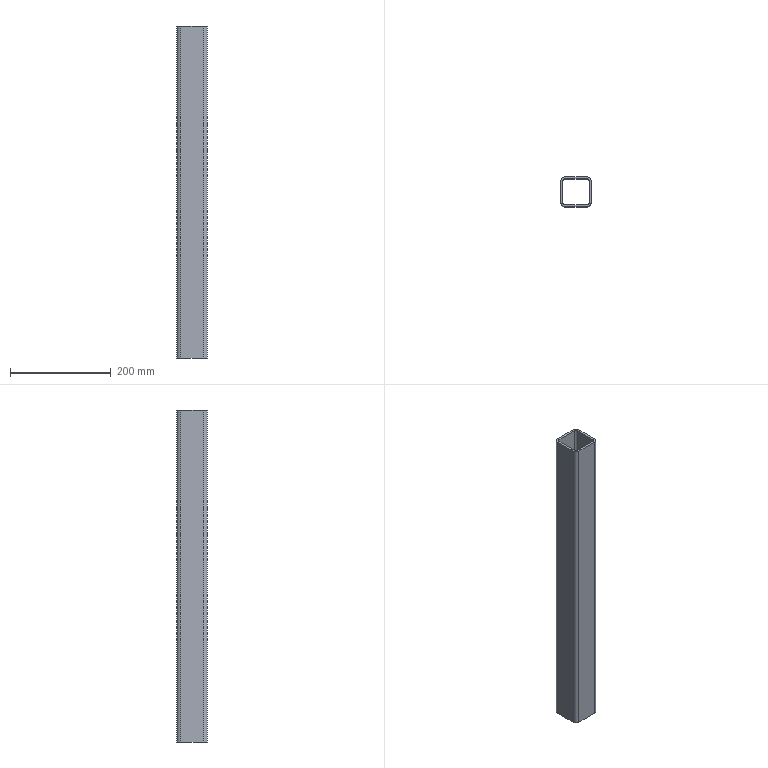Part | SolidWorks | features BaseBody 1 | 1 solid | 18 faces | box 60 x 60 x 660 mm | volume 564166 mm3 | plane 10 | cylinder 8 | commonest cylinder face diameters 8 x4 16 x4
STEP:
#1=CARTESIAN_POINT('',(126.,0.,-60.));
#2=VERTEX_POINT('',#1);
#3=CARTESIAN_POINT('',(126.,44.,-60.));
#4=VERTEX_POINT('',#3);
#5=CARTESIAN_POINT('',(126.,44.,-60.));
#6=DIRECTION('',(0.,1.,0.));
#7=VECTOR('',#6,1000.);
#8=LINE('',#5,#7);
#9=EDGE_CURVE('',#2,#4,#8,.T.);
#10=ORIENTED_EDGE('',*,*,#9,.T.);
#11=CARTESIAN_POINT('',(126.,44.,-720.));
#12=VERTEX_POINT('',#11);
#13=CARTESIAN_POINT('',(126.,44.,-1270.));
#14=DIRECTION('',(0.,0.,-1.));
#15=VECTOR('',#14,1000.);
#16=LINE('',#13,#15);
#17=EDGE_CURVE('',#4,#12,#16,.T.);
#18=ORIENTED_EDGE('',*,*,#17,.T.);
#19=CARTESIAN_POINT('',(126.,0.,-720.));
#20=VERTEX_POINT('',#19);
#21=CARTESIAN_POINT('',(126.,44.,-720.));
#22=DIRECTION('',(0.,-1.,0.));
#23=VECTOR('',#22,1000.);
#24=LINE('',#21,#23);
#25=EDGE_CURVE('',#12,#20,#24,.T.);
#26=ORIENTED_EDGE('',*,*,#25,.T.);
#27=CARTESIAN_POINT('',(126.,0.,-1270.));
#28=DIRECTION('',(0.,0.,1.));
#29=VECTOR('',#28,1000.);
#30=LINE('',#27,#29);
#31=EDGE_CURVE('',#20,#2,#30,.T.);
#32=ORIENTED_EDGE('',*,*,#31,.T.);
#33=EDGE_LOOP('',(#10,#18,#26,#32));
#34=FACE_OUTER_BOUND('',#33,.T.);
#35=CARTESIAN_POINT('',(126.,44.,-1270.));
#36=DIRECTION('',(-1.,0.,0.));
#37=DIRECTION('',(0.,0.,1.));
#38=AXIS2_PLACEMENT_3D('',#35,#36,#37);
#39=PLANE('',#38);
#40=ADVANCED_FACE('',(#34),#39,.T.);
#41=ORIENTED_EDGE('',*,*,#17,.F.);
#42=CARTESIAN_POINT('',(122.,48.,-60.));
#43=VERTEX_POINT('',#42);
#44=CARTESIAN_POINT('',(122.,44.,-60.));
#45=DIRECTION('',(0.,0.,-1.));
#46=DIRECTION('',(1.,0.,0.));
#47=AXIS2_PLACEMENT_3D('',#44,#45,#46);
#48=CIRCLE('',#47,4.);
#49=EDGE_CURVE('',#43,#4,#48,.T.);
#50=ORIENTED_EDGE('',*,*,#49,.F.);
#51=CARTESIAN_POINT('',(122.,48.,-720.));
#52=VERTEX_POINT('',#51);
#53=CARTESIAN_POINT('',(122.,48.,-1270.));
#54=DIRECTION('',(0.,0.,1.));
#55=VECTOR('',#54,1000.);
#56=LINE('',#53,#55);
#57=EDGE_CURVE('',#52,#43,#56,.T.);
#58=ORIENTED_EDGE('',*,*,#57,.F.);
#59=CARTESIAN_POINT('',(122.,44.,-720.));
#60=DIRECTION('',(0.,0.,1.));
#61=DIRECTION('',(1.,0.,0.));
#62=AXIS2_PLACEMENT_3D('',#59,#60,#61);
#63=CIRCLE('',#62,4.);
#64=EDGE_CURVE('',#12,#52,#63,.T.);
#65=ORIENTED_EDGE('',*,*,#64,.F.);
#66=EDGE_LOOP('',(#41,#50,#58,#65));
#67=FACE_OUTER_BOUND('',#66,.T.);
#68=CARTESIAN_POINT('',(122.,44.,-1270.));
#69=DIRECTION('',(0.,0.,1.));
#70=DIRECTION('',(1.,0.,0.));
#71=AXIS2_PLACEMENT_3D('',#68,#69,#70);
#72=CYLINDRICAL_SURFACE('',#71,4.);
#73=ADVANCED_FACE('',(#67),#72,.F.);
#74=CARTESIAN_POINT('',(122.,-4.,-60.));
#75=VERTEX_POINT('',#74);
#76=CARTESIAN_POINT('',(122.,0.,-60.));
#77=DIRECTION('',(0.,0.,-1.));
#78=DIRECTION('',(1.,0.,0.));
#79=AXIS2_PLACEMENT_3D('',#76,#77,#78);
#80=CIRCLE('',#79,4.);
#81=EDGE_CURVE('',#2,#75,#80,.T.);
#82=ORIENTED_EDGE('',*,*,#81,.T.);
#83=CARTESIAN_POINT('',(78.,-4.,-60.));
#84=VERTEX_POINT('',#83);
#85=CARTESIAN_POINT('',(670.,-4.,-60.));
#86=DIRECTION('',(-1.,0.,0.));
#87=VECTOR('',#86,1000.);
#88=LINE('',#85,#87);
#89=EDGE_CURVE('',#75,#84,#88,.T.);
#90=ORIENTED_EDGE('',*,*,#89,.T.);
#91=CARTESIAN_POINT('',(74.,0.,-60.));
#92=VERTEX_POINT('',#91);
#93=CARTESIAN_POINT('',(78.,0.,-60.));
#94=DIRECTION('',(0.,0.,-1.));
#95=DIRECTION('',(1.,0.,0.));
#96=AXIS2_PLACEMENT_3D('',#93,#94,#95);
#97=CIRCLE('',#96,4.);
#98=EDGE_CURVE('',#84,#92,#97,.T.);
#99=ORIENTED_EDGE('',*,*,#98,.T.);
#100=CARTESIAN_POINT('',(74.,44.,-60.));
#101=VERTEX_POINT('',#100);
#102=CARTESIAN_POINT('',(74.,0.,-60.));
#103=DIRECTION('',(0.,1.,0.));
#104=VECTOR('',#103,1000.);
#105=LINE('',#102,#104);
#106=EDGE_CURVE('',#92,#101,#105,.T.);
#107=ORIENTED_EDGE('',*,*,#106,.T.);
#108=CARTESIAN_POINT('',(78.,48.,-60.));
#109=VERTEX_POINT('',#108);
#110=CARTESIAN_POINT('',(78.,44.,-60.));
#111=DIRECTION('',(0.,0.,-1.));
#112=DIRECTION('',(1.,0.,0.));
#113=AXIS2_PLACEMENT_3D('',#110,#111,#112);
#114=CIRCLE('',#113,4.);
#115=EDGE_CURVE('',#101,#109,#114,.T.);
#116=ORIENTED_EDGE('',*,*,#115,.T.);
#117=CARTESIAN_POINT('',(670.,48.,-60.));
#118=DIRECTION('',(1.,0.,0.));
#119=VECTOR('',#118,1000.);
#120=LINE('',#117,#119);
#121=EDGE_CURVE('',#109,#43,#120,.T.);
#122=ORIENTED_EDGE('',*,*,#121,.T.);
#123=ORIENTED_EDGE('',*,*,#49,.T.);
#124=ORIENTED_EDGE('',*,*,#9,.F.);
#125=EDGE_LOOP('',(#82,#90,#99,#107,#116,#122,#123,#124));
#126=FACE_BOUND('',#125,.T.);
#127=CARTESIAN_POINT('',(130.,0.,-60.));
#128=VERTEX_POINT('',#127);
#129=CARTESIAN_POINT('',(130.,44.,-60.));
#130=VERTEX_POINT('',#129);
#131=CARTESIAN_POINT('',(130.,0.,-60.));
#132=DIRECTION('',(0.,1.,0.));
#133=VECTOR('',#132,1000.);
#134=LINE('',#131,#133);
#135=EDGE_CURVE('',#128,#130,#134,.T.);
#136=ORIENTED_EDGE('',*,*,#135,.T.);
#137=CARTESIAN_POINT('',(122.,52.,-60.));
#138=VERTEX_POINT('',#137);
#139=CARTESIAN_POINT('',(122.,44.,-60.));
#140=DIRECTION('',(0.,0.,1.));
#141=DIRECTION('',(1.,0.,0.));
#142=AXIS2_PLACEMENT_3D('',#139,#140,#141);
#143=CIRCLE('',#142,8.);
#144=EDGE_CURVE('',#130,#138,#143,.T.);
#145=ORIENTED_EDGE('',*,*,#144,.T.);
#146=CARTESIAN_POINT('',(78.,52.,-60.));
#147=VERTEX_POINT('',#146);
#148=CARTESIAN_POINT('',(670.,52.,-60.));
#149=DIRECTION('',(-1.,0.,0.));
#150=VECTOR('',#149,1000.);
#151=LINE('',#148,#150);
#152=EDGE_CURVE('',#138,#147,#151,.T.);
#153=ORIENTED_EDGE('',*,*,#152,.T.);
#154=CARTESIAN_POINT('',(70.,44.,-60.));
#155=VERTEX_POINT('',#154);
#156=CARTESIAN_POINT('',(78.,44.,-60.));
#157=DIRECTION('',(0.,0.,1.));
#158=DIRECTION('',(1.,0.,0.));
#159=AXIS2_PLACEMENT_3D('',#156,#157,#158);
#160=CIRCLE('',#159,8.);
#161=EDGE_CURVE('',#147,#155,#160,.T.);
#162=ORIENTED_EDGE('',*,*,#161,.T.);
#163=CARTESIAN_POINT('',(70.,0.,-60.));
#164=VERTEX_POINT('',#163);
#165=CARTESIAN_POINT('',(70.,0.,-60.));
#166=DIRECTION('',(0.,-1.,0.));
#167=VECTOR('',#166,1000.);
#168=LINE('',#165,#167);
#169=EDGE_CURVE('',#155,#164,#168,.T.);
#170=ORIENTED_EDGE('',*,*,#169,.T.);
#171=CARTESIAN_POINT('',(78.,-8.,-60.));
#172=VERTEX_POINT('',#171);
#173=CARTESIAN_POINT('',(78.,0.,-60.));
#174=DIRECTION('',(0.,0.,1.));
#175=DIRECTION('',(1.,0.,0.));
#176=AXIS2_PLACEMENT_3D('',#173,#174,#175);
#177=CIRCLE('',#176,8.);
#178=EDGE_CURVE('',#164,#172,#177,.T.);
#179=ORIENTED_EDGE('',*,*,#178,.T.);
#180=CARTESIAN_POINT('',(122.,-8.,-60.));
#181=VERTEX_POINT('',#180);
#182=CARTESIAN_POINT('',(670.,-8.,-60.));
#183=DIRECTION('',(1.,0.,0.));
#184=VECTOR('',#183,1000.);
#185=LINE('',#182,#184);
#186=EDGE_CURVE('',#172,#181,#185,.T.);
#187=ORIENTED_EDGE('',*,*,#186,.T.);
#188=CARTESIAN_POINT('',(122.,0.,-60.));
#189=DIRECTION('',(0.,0.,1.));
#190=DIRECTION('',(1.,0.,0.));
#191=AXIS2_PLACEMENT_3D('',#188,#189,#190);
#192=CIRCLE('',#191,8.);
#193=EDGE_CURVE('',#181,#128,#192,.T.);
#194=ORIENTED_EDGE('',*,*,#193,.T.);
#195=EDGE_LOOP('',(#136,#145,#153,#162,#170,#179,#187,#194));
#196=FACE_OUTER_BOUND('',#195,.T.);
#197=CARTESIAN_POINT('',(670.,0.,-60.));
#198=DIRECTION('',(0.,0.,1.));
#199=DIRECTION('',(1.,0.,0.));
#200=AXIS2_PLACEMENT_3D('',#197,#198,#199);
#201=PLANE('',#200);
#202=ADVANCED_FACE('',(#126,#196),#201,.T.);
#203=CARTESIAN_POINT('',(122.,-4.,-720.));
#204=VERTEX_POINT('',#203);
#205=CARTESIAN_POINT('',(122.,-4.,-1270.));
#206=DIRECTION('',(0.,0.,-1.));
#207=VECTOR('',#206,1000.);
#208=LINE('',#205,#207);
#209=EDGE_CURVE('',#75,#204,#208,.T.);
#210=ORIENTED_EDGE('',*,*,#209,.F.);
#211=ORIENTED_EDGE('',*,*,#81,.F.);
#212=ORIENTED_EDGE('',*,*,#31,.F.);
#213=CARTESIAN_POINT('',(122.,0.,-720.));
#214=DIRECTION('',(0.,0.,1.));
#215=DIRECTION('',(1.,0.,0.));
#216=AXIS2_PLACEMENT_3D('',#213,#214,#215);
#217=CIRCLE('',#216,4.);
#218=EDGE_CURVE('',#204,#20,#217,.T.);
#219=ORIENTED_EDGE('',*,*,#218,.F.);
#220=EDGE_LOOP('',(#210,#211,#212,#219));
#221=FACE_OUTER_BOUND('',#220,.T.);
#222=CARTESIAN_POINT('',(122.,0.,-1270.));
#223=DIRECTION('',(0.,0.,1.));
#224=DIRECTION('',(1.,0.,0.));
#225=AXIS2_PLACEMENT_3D('',#222,#223,#224);
#226=CYLINDRICAL_SURFACE('',#225,4.);
#227=ADVANCED_FACE('',(#221),#226,.F.);
#228=CARTESIAN_POINT('',(78.,-4.,-720.));
#229=VERTEX_POINT('',#228);
#230=CARTESIAN_POINT('',(0.,-4.,-720.));
#231=DIRECTION('',(1.,0.,0.));
#232=VECTOR('',#231,1000.);
#233=LINE('',#230,#232);
#234=EDGE_CURVE('',#229,#204,#233,.T.);
#235=ORIENTED_EDGE('',*,*,#234,.T.);
#236=ORIENTED_EDGE('',*,*,#218,.T.);
#237=ORIENTED_EDGE('',*,*,#25,.F.);
#238=ORIENTED_EDGE('',*,*,#64,.T.);
#239=CARTESIAN_POINT('',(78.,48.,-720.));
#240=VERTEX_POINT('',#239);
#241=CARTESIAN_POINT('',(0.,48.,-720.));
#242=DIRECTION('',(-1.,0.,0.));
#243=VECTOR('',#242,1000.);
#244=LINE('',#241,#243);
#245=EDGE_CURVE('',#52,#240,#244,.T.);
#246=ORIENTED_EDGE('',*,*,#245,.T.);
#247=CARTESIAN_POINT('',(74.,44.,-720.));
#248=VERTEX_POINT('',#247);
#249=CARTESIAN_POINT('',(78.,44.,-720.));
#250=DIRECTION('',(0.,0.,1.));
#251=DIRECTION('',(1.,0.,0.));
#252=AXIS2_PLACEMENT_3D('',#249,#250,#251);
#253=CIRCLE('',#252,4.);
#254=EDGE_CURVE('',#240,#248,#253,.T.);
#255=ORIENTED_EDGE('',*,*,#254,.T.);
#256=CARTESIAN_POINT('',(74.,0.,-720.));
#257=VERTEX_POINT('',#256);
#258=CARTESIAN_POINT('',(74.,1242.,-720.));
#259=DIRECTION('',(0.,-1.,0.));
#260=VECTOR('',#259,1000.);
#261=LINE('',#258,#260);
#262=EDGE_CURVE('',#248,#257,#261,.T.);
#263=ORIENTED_EDGE('',*,*,#262,.T.);
#264=CARTESIAN_POINT('',(78.,0.,-720.));
#265=DIRECTION('',(0.,0.,1.));
#266=DIRECTION('',(1.,0.,0.));
#267=AXIS2_PLACEMENT_3D('',#264,#265,#266);
#268=CIRCLE('',#267,4.);
#269=EDGE_CURVE('',#257,#229,#268,.T.);
#270=ORIENTED_EDGE('',*,*,#269,.T.);
#271=EDGE_LOOP('',(#235,#236,#237,#238,#246,#255,#263,#270));
#272=FACE_BOUND('',#271,.T.);
#273=CARTESIAN_POINT('',(70.,44.,-720.));
#274=VERTEX_POINT('',#273);
#275=CARTESIAN_POINT('',(78.,52.,-720.));
#276=VERTEX_POINT('',#275);
#277=CARTESIAN_POINT('',(78.,44.,-720.));
#278=DIRECTION('',(0.,0.,-1.));
#279=DIRECTION('',(1.,0.,0.));
#280=AXIS2_PLACEMENT_3D('',#277,#278,#279);
#281=CIRCLE('',#280,8.);
#282=EDGE_CURVE('',#274,#276,#281,.T.);
#283=ORIENTED_EDGE('',*,*,#282,.T.);
#284=CARTESIAN_POINT('',(122.,52.,-720.));
#285=VERTEX_POINT('',#284);
#286=CARTESIAN_POINT('',(0.,52.,-720.));
#287=DIRECTION('',(1.,0.,0.));
#288=VECTOR('',#287,1000.);
#289=LINE('',#286,#288);
#290=EDGE_CURVE('',#276,#285,#289,.T.);
#291=ORIENTED_EDGE('',*,*,#290,.T.);
#292=CARTESIAN_POINT('',(130.,44.,-720.));
#293=VERTEX_POINT('',#292);
#294=CARTESIAN_POINT('',(122.,44.,-720.));
#295=DIRECTION('',(0.,0.,-1.));
#296=DIRECTION('',(1.,0.,0.));
#297=AXIS2_PLACEMENT_3D('',#294,#295,#296);
#298=CIRCLE('',#297,8.);
#299=EDGE_CURVE('',#285,#293,#298,.T.);
#300=ORIENTED_EDGE('',*,*,#299,.T.);
#301=CARTESIAN_POINT('',(130.,0.,-720.));
#302=VERTEX_POINT('',#301);
#303=CARTESIAN_POINT('',(130.,1242.,-720.));
#304=DIRECTION('',(0.,-1.,0.));
#305=VECTOR('',#304,1000.);
#306=LINE('',#303,#305);
#307=EDGE_CURVE('',#293,#302,#306,.T.);
#308=ORIENTED_EDGE('',*,*,#307,.T.);
#309=CARTESIAN_POINT('',(122.,-8.,-720.));
#310=VERTEX_POINT('',#309);
#311=CARTESIAN_POINT('',(122.,0.,-720.));
#312=DIRECTION('',(0.,0.,-1.));
#313=DIRECTION('',(1.,0.,0.));
#314=AXIS2_PLACEMENT_3D('',#311,#312,#313);
#315=CIRCLE('',#314,8.);
#316=EDGE_CURVE('',#302,#310,#315,.T.);
#317=ORIENTED_EDGE('',*,*,#316,.T.);
#318=CARTESIAN_POINT('',(78.,-8.,-720.));
#319=VERTEX_POINT('',#318);
#320=CARTESIAN_POINT('',(0.,-8.,-720.));
#321=DIRECTION('',(-1.,0.,0.));
#322=VECTOR('',#321,1000.);
#323=LINE('',#320,#322);
#324=EDGE_CURVE('',#310,#319,#323,.T.);
#325=ORIENTED_EDGE('',*,*,#324,.T.);
#326=CARTESIAN_POINT('',(70.,0.,-720.));
#327=VERTEX_POINT('',#326);
#328=CARTESIAN_POINT('',(78.,0.,-720.));
#329=DIRECTION('',(0.,0.,-1.));
#330=DIRECTION('',(1.,0.,0.));
#331=AXIS2_PLACEMENT_3D('',#328,#329,#330);
#332=CIRCLE('',#331,8.);
#333=EDGE_CURVE('',#319,#327,#332,.T.);
#334=ORIENTED_EDGE('',*,*,#333,.T.);
#335=CARTESIAN_POINT('',(70.,1242.,-720.));
#336=DIRECTION('',(0.,1.,0.));
#337=VECTOR('',#336,1000.);
#338=LINE('',#335,#337);
#339=EDGE_CURVE('',#327,#274,#338,.T.);
#340=ORIENTED_EDGE('',*,*,#339,.T.);
#341=EDGE_LOOP('',(#283,#291,#300,#308,#317,#325,#334,#340));
#342=FACE_OUTER_BOUND('',#341,.T.);
#343=CARTESIAN_POINT('',(0.,1242.,-720.));
#344=DIRECTION('',(0.,0.,-1.));
#345=DIRECTION('',(-1.,0.,0.));
#346=AXIS2_PLACEMENT_3D('',#343,#344,#345);
#347=PLANE('',#346);
#348=ADVANCED_FACE('',(#272,#342),#347,.T.);
#349=ORIENTED_EDGE('',*,*,#121,.F.);
#350=CARTESIAN_POINT('',(78.,48.,-1270.));
#351=DIRECTION('',(0.,0.,-1.));
#352=VECTOR('',#351,1000.);
#353=LINE('',#350,#352);
#354=EDGE_CURVE('',#109,#240,#353,.T.);
#355=ORIENTED_EDGE('',*,*,#354,.T.);
#356=ORIENTED_EDGE('',*,*,#245,.F.);
#357=ORIENTED_EDGE('',*,*,#57,.T.);
#358=EDGE_LOOP('',(#349,#355,#356,#357));
#359=FACE_OUTER_BOUND('',#358,.T.);
#360=CARTESIAN_POINT('',(122.,48.,-1270.));
#361=DIRECTION('',(0.,-1.,0.));
#362=DIRECTION('',(0.,0.,-1.));
#363=AXIS2_PLACEMENT_3D('',#360,#361,#362);
#364=PLANE('',#363);
#365=ADVANCED_FACE('',(#359),#364,.T.);
#366=ORIENTED_EDGE('',*,*,#89,.F.);
#367=ORIENTED_EDGE('',*,*,#209,.T.);
#368=ORIENTED_EDGE('',*,*,#234,.F.);
#369=CARTESIAN_POINT('',(78.,-4.,-1270.));
#370=DIRECTION('',(0.,0.,1.));
#371=VECTOR('',#370,1000.);
#372=LINE('',#369,#371);
#373=EDGE_CURVE('',#229,#84,#372,.T.);
#374=ORIENTED_EDGE('',*,*,#373,.T.);
#375=EDGE_LOOP('',(#366,#367,#368,#374));
#376=FACE_OUTER_BOUND('',#375,.T.);
#377=CARTESIAN_POINT('',(78.,-4.,-1270.));
#378=DIRECTION('',(0.,1.,0.));
#379=DIRECTION('',(0.,0.,1.));
#380=AXIS2_PLACEMENT_3D('',#377,#378,#379);
#381=PLANE('',#380);
#382=ADVANCED_FACE('',(#376),#381,.T.);
#383=ORIENTED_EDGE('',*,*,#354,.F.);
#384=ORIENTED_EDGE('',*,*,#115,.F.);
#385=CARTESIAN_POINT('',(74.,44.,-1270.));
#386=DIRECTION('',(0.,0.,1.));
#387=VECTOR('',#386,1000.);
#388=LINE('',#385,#387);
#389=EDGE_CURVE('',#248,#101,#388,.T.);
#390=ORIENTED_EDGE('',*,*,#389,.F.);
#391=ORIENTED_EDGE('',*,*,#254,.F.);
#392=EDGE_LOOP('',(#383,#384,#390,#391));
#393=FACE_OUTER_BOUND('',#392,.T.);
#394=CARTESIAN_POINT('',(78.,44.,-1270.));
#395=DIRECTION('',(0.,0.,1.));
#396=DIRECTION('',(1.,0.,0.));
#397=AXIS2_PLACEMENT_3D('',#394,#395,#396);
#398=CYLINDRICAL_SURFACE('',#397,4.);
#399=ADVANCED_FACE('',(#393),#398,.F.);
#400=ORIENTED_EDGE('',*,*,#106,.F.);
#401=CARTESIAN_POINT('',(74.,0.,-1270.));
#402=DIRECTION('',(0.,0.,-1.));
#403=VECTOR('',#402,1000.);
#404=LINE('',#401,#403);
#405=EDGE_CURVE('',#92,#257,#404,.T.);
#406=ORIENTED_EDGE('',*,*,#405,.T.);
#407=ORIENTED_EDGE('',*,*,#262,.F.);
#408=ORIENTED_EDGE('',*,*,#389,.T.);
#409=EDGE_LOOP('',(#400,#406,#407,#408));
#410=FACE_OUTER_BOUND('',#409,.T.);
#411=CARTESIAN_POINT('',(74.,0.,-1270.));
#412=DIRECTION('',(1.,0.,0.));
#413=DIRECTION('',(0.,0.,-1.));
#414=AXIS2_PLACEMENT_3D('',#411,#412,#413);
#415=PLANE('',#414);
#416=ADVANCED_FACE('',(#410),#415,.T.);
#417=ORIENTED_EDGE('',*,*,#405,.F.);
#418=ORIENTED_EDGE('',*,*,#98,.F.);
#419=ORIENTED_EDGE('',*,*,#373,.F.);
#420=ORIENTED_EDGE('',*,*,#269,.F.);
#421=EDGE_LOOP('',(#417,#418,#419,#420));
#422=FACE_OUTER_BOUND('',#421,.T.);
#423=CARTESIAN_POINT('',(78.,0.,-1270.));
#424=DIRECTION('',(0.,0.,1.));
#425=DIRECTION('',(1.,0.,0.));
#426=AXIS2_PLACEMENT_3D('',#423,#424,#425);
#427=CYLINDRICAL_SURFACE('',#426,4.);
#428=ADVANCED_FACE('',(#422),#427,.F.);
#429=CARTESIAN_POINT('',(130.,44.,-1270.));
#430=DIRECTION('',(0.,0.,-1.));
#431=VECTOR('',#430,1000.);
#432=LINE('',#429,#431);
#433=EDGE_CURVE('',#130,#293,#432,.T.);
#434=ORIENTED_EDGE('',*,*,#433,.T.);
#435=ORIENTED_EDGE('',*,*,#299,.F.);
#436=CARTESIAN_POINT('',(122.,52.,-1270.));
#437=DIRECTION('',(0.,0.,1.));
#438=VECTOR('',#437,1000.);
#439=LINE('',#436,#438);
#440=EDGE_CURVE('',#285,#138,#439,.T.);
#441=ORIENTED_EDGE('',*,*,#440,.T.);
#442=ORIENTED_EDGE('',*,*,#144,.F.);
#443=EDGE_LOOP('',(#434,#435,#441,#442));
#444=FACE_OUTER_BOUND('',#443,.T.);
#445=CARTESIAN_POINT('',(122.,44.,-1270.));
#446=DIRECTION('',(0.,0.,1.));
#447=DIRECTION('',(1.,0.,0.));
#448=AXIS2_PLACEMENT_3D('',#445,#446,#447);
#449=CYLINDRICAL_SURFACE('',#448,8.);
#450=ADVANCED_FACE('',(#444),#449,.T.);
#451=ORIENTED_EDGE('',*,*,#135,.F.);
#452=CARTESIAN_POINT('',(130.,0.,-1270.));
#453=DIRECTION('',(0.,0.,1.));
#454=VECTOR('',#453,1000.);
#455=LINE('',#452,#454);
#456=EDGE_CURVE('',#302,#128,#455,.T.);
#457=ORIENTED_EDGE('',*,*,#456,.F.);
#458=ORIENTED_EDGE('',*,*,#307,.F.);
#459=ORIENTED_EDGE('',*,*,#433,.F.);
#460=EDGE_LOOP('',(#451,#457,#458,#459));
#461=FACE_OUTER_BOUND('',#460,.T.);
#462=CARTESIAN_POINT('',(130.,44.,-1270.));
#463=DIRECTION('',(-1.,0.,0.));
#464=DIRECTION('',(0.,0.,1.));
#465=AXIS2_PLACEMENT_3D('',#462,#463,#464);
#466=PLANE('',#465);
#467=ADVANCED_FACE('',(#461),#466,.F.);
#468=CARTESIAN_POINT('',(122.,-8.,-1270.));
#469=DIRECTION('',(0.,0.,-1.));
#470=VECTOR('',#469,1000.);
#471=LINE('',#468,#470);
#472=EDGE_CURVE('',#181,#310,#471,.T.);
#473=ORIENTED_EDGE('',*,*,#472,.T.);
#474=ORIENTED_EDGE('',*,*,#316,.F.);
#475=ORIENTED_EDGE('',*,*,#456,.T.);
#476=ORIENTED_EDGE('',*,*,#193,.F.);
#477=EDGE_LOOP('',(#473,#474,#475,#476));
#478=FACE_OUTER_BOUND('',#477,.T.);
#479=CARTESIAN_POINT('',(122.,0.,-1270.));
#480=DIRECTION('',(0.,0.,1.));
#481=DIRECTION('',(1.,0.,0.));
#482=AXIS2_PLACEMENT_3D('',#479,#480,#481);
#483=CYLINDRICAL_SURFACE('',#482,8.);
#484=ADVANCED_FACE('',(#478),#483,.T.);
#485=ORIENTED_EDGE('',*,*,#186,.F.);
#486=CARTESIAN_POINT('',(78.,-8.,-1270.));
#487=DIRECTION('',(0.,0.,1.));
#488=VECTOR('',#487,1000.);
#489=LINE('',#486,#488);
#490=EDGE_CURVE('',#319,#172,#489,.T.);
#491=ORIENTED_EDGE('',*,*,#490,.F.);
#492=ORIENTED_EDGE('',*,*,#324,.F.);
#493=ORIENTED_EDGE('',*,*,#472,.F.);
#494=EDGE_LOOP('',(#485,#491,#492,#493));
#495=FACE_OUTER_BOUND('',#494,.T.);
#496=CARTESIAN_POINT('',(78.,-8.,-1270.));
#497=DIRECTION('',(0.,1.,0.));
#498=DIRECTION('',(0.,0.,1.));
#499=AXIS2_PLACEMENT_3D('',#496,#497,#498);
#500=PLANE('',#499);
#501=ADVANCED_FACE('',(#495),#500,.F.);
#502=CARTESIAN_POINT('',(70.,0.,-1270.));
#503=DIRECTION('',(0.,0.,-1.));
#504=VECTOR('',#503,1000.);
#505=LINE('',#502,#504);
#506=EDGE_CURVE('',#164,#327,#505,.T.);
#507=ORIENTED_EDGE('',*,*,#506,.T.);
#508=ORIENTED_EDGE('',*,*,#333,.F.);
#509=ORIENTED_EDGE('',*,*,#490,.T.);
#510=ORIENTED_EDGE('',*,*,#178,.F.);
#511=EDGE_LOOP('',(#507,#508,#509,#510));
#512=FACE_OUTER_BOUND('',#511,.T.);
#513=CARTESIAN_POINT('',(78.,0.,-1270.));
#514=DIRECTION('',(0.,0.,1.));
#515=DIRECTION('',(1.,0.,0.));
#516=AXIS2_PLACEMENT_3D('',#513,#514,#515);
#517=CYLINDRICAL_SURFACE('',#516,8.);
#518=ADVANCED_FACE('',(#512),#517,.T.);
#519=ORIENTED_EDGE('',*,*,#169,.F.);
#520=CARTESIAN_POINT('',(70.,44.,-1270.));
#521=DIRECTION('',(0.,0.,1.));
#522=VECTOR('',#521,1000.);
#523=LINE('',#520,#522);
#524=EDGE_CURVE('',#274,#155,#523,.T.);
#525=ORIENTED_EDGE('',*,*,#524,.F.);
#526=ORIENTED_EDGE('',*,*,#339,.F.);
#527=ORIENTED_EDGE('',*,*,#506,.F.);
#528=EDGE_LOOP('',(#519,#525,#526,#527));
#529=FACE_OUTER_BOUND('',#528,.T.);
#530=CARTESIAN_POINT('',(70.,0.,-1270.));
#531=DIRECTION('',(1.,0.,0.));
#532=DIRECTION('',(0.,0.,-1.));
#533=AXIS2_PLACEMENT_3D('',#530,#531,#532);
#534=PLANE('',#533);
#535=ADVANCED_FACE('',(#529),#534,.F.);
#536=CARTESIAN_POINT('',(78.,52.,-1270.));
#537=DIRECTION('',(0.,0.,-1.));
#538=VECTOR('',#537,1000.);
#539=LINE('',#536,#538);
#540=EDGE_CURVE('',#147,#276,#539,.T.);
#541=ORIENTED_EDGE('',*,*,#540,.T.);
#542=ORIENTED_EDGE('',*,*,#282,.F.);
#543=ORIENTED_EDGE('',*,*,#524,.T.);
#544=ORIENTED_EDGE('',*,*,#161,.F.);
#545=EDGE_LOOP('',(#541,#542,#543,#544));
#546=FACE_OUTER_BOUND('',#545,.T.);
#547=CARTESIAN_POINT('',(78.,44.,-1270.));
#548=DIRECTION('',(0.,0.,1.));
#549=DIRECTION('',(1.,0.,0.));
#550=AXIS2_PLACEMENT_3D('',#547,#548,#549);
#551=CYLINDRICAL_SURFACE('',#550,8.);
#552=ADVANCED_FACE('',(#546),#551,.T.);
#553=ORIENTED_EDGE('',*,*,#152,.F.);
#554=ORIENTED_EDGE('',*,*,#440,.F.);
#555=ORIENTED_EDGE('',*,*,#290,.F.);
#556=ORIENTED_EDGE('',*,*,#540,.F.);
#557=EDGE_LOOP('',(#553,#554,#555,#556));
#558=FACE_OUTER_BOUND('',#557,.T.);
#559=CARTESIAN_POINT('',(122.,52.,-1270.));
#560=DIRECTION('',(0.,-1.,0.));
#561=DIRECTION('',(0.,0.,-1.));
#562=AXIS2_PLACEMENT_3D('',#559,#560,#561);
#563=PLANE('',#562);
#564=ADVANCED_FACE('',(#558),#563,.F.);
#565=CLOSED_SHELL('',(#40,#73,#202,#227,#348,#365,#382,#399,#416,#428,#450,#467,#484,#501,#518,#535,#552,#564));
#566=MANIFOLD_SOLID_BREP('',#565);
#567=CARTESIAN_POINT('',(0.,0.,0.));
#568=DIRECTION('',(0.,0.,1.));
#569=DIRECTION('',(1.,0.,0.));
#570=AXIS2_PLACEMENT_3D('',#567,#568,#569);
#571=(LENGTH_UNIT()NAMED_UNIT(*)SI_UNIT(.MILLI.,.METRE.));
#572=UNCERTAINTY_MEASURE_WITH_UNIT(LENGTH_MEASURE(0.00001),#571,'','');
#573=(NAMED_UNIT(*)PLANE_ANGLE_UNIT()SI_UNIT($,.RADIAN.));
#574=(NAMED_UNIT(*)SI_UNIT($,.STERADIAN.)SOLID_ANGLE_UNIT());
#575=(GEOMETRIC_REPRESENTATION_CONTEXT(3)GLOBAL_UNCERTAINTY_ASSIGNED_CONTEXT((#572))GLOBAL_UNIT_ASSIGNED_CONTEXT((#571,#573,#574))REPRESENTATION_CONTEXT('',''));
#576=ADVANCED_BREP_SHAPE_REPRESENTATION('',(#566,#570),#575);